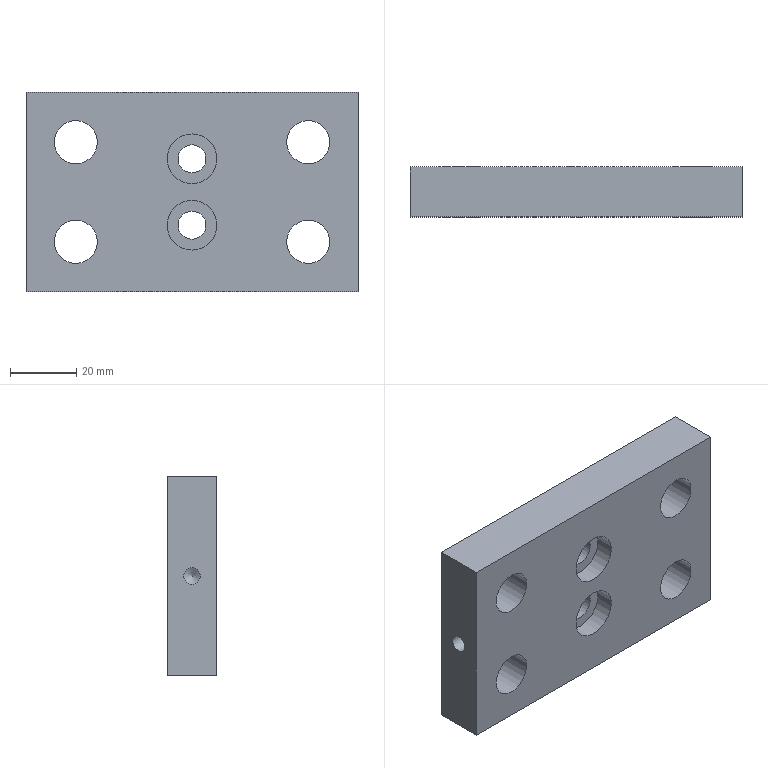Part | NX | features BREP 1 | 1 solid | 26 faces | box 100 x 15 x 60 mm | volume 77616 mm3 | cylinder 13 | plane 8 | cone 5 | commonest cylinder face diameters 13 x4 5 x3 6 x2 8.4 x2 15 x2
STEP:
#1=CARTESIAN_POINT('',(50.,-7.5,30.));
#2=VERTEX_POINT('',#1);
#3=CARTESIAN_POINT('',(50.,-7.5,-30.));
#4=VERTEX_POINT('',#3);
#5=CARTESIAN_POINT('',(50.,-7.5,30.));
#6=DIRECTION('',(0.,0.,-1.));
#7=VECTOR('',#6,1000.);
#8=LINE('',#5,#7);
#9=EDGE_CURVE('',#2,#4,#8,.T.);
#10=ORIENTED_EDGE('',*,*,#9,.T.);
#11=CARTESIAN_POINT('',(50.,7.5,-30.));
#12=VERTEX_POINT('',#11);
#13=CARTESIAN_POINT('',(50.,7.5,-30.));
#14=DIRECTION('',(0.,-1.,0.));
#15=VECTOR('',#14,1000.);
#16=LINE('',#13,#15);
#17=EDGE_CURVE('',#12,#4,#16,.T.);
#18=ORIENTED_EDGE('',*,*,#17,.F.);
#19=CARTESIAN_POINT('',(50.,7.5,30.));
#20=VERTEX_POINT('',#19);
#21=CARTESIAN_POINT('',(50.,7.5,30.));
#22=DIRECTION('',(0.,0.,-1.));
#23=VECTOR('',#22,1000.);
#24=LINE('',#21,#23);
#25=EDGE_CURVE('',#20,#12,#24,.T.);
#26=ORIENTED_EDGE('',*,*,#25,.F.);
#27=CARTESIAN_POINT('',(50.,7.5,30.));
#28=DIRECTION('',(0.,-1.,0.));
#29=VECTOR('',#28,1000.);
#30=LINE('',#27,#29);
#31=EDGE_CURVE('',#20,#2,#30,.T.);
#32=ORIENTED_EDGE('',*,*,#31,.T.);
#33=EDGE_LOOP('',(#10,#18,#26,#32));
#34=FACE_BOUND('',#33,.T.);
#35=CARTESIAN_POINT('',(50.,7.5,30.));
#36=DIRECTION('',(-1.,0.,0.));
#37=DIRECTION('',(0.,0.,-1.));
#38=AXIS2_PLACEMENT_3D('',#35,#36,#37);
#39=PLANE('',#38);
#40=ADVANCED_FACE('',(#34),#39,.F.);
#41=CARTESIAN_POINT('',(-27.5,0.,-30.));
#42=VERTEX_POINT('',#41);
#43=CARTESIAN_POINT('',(-25.,0.,-30.));
#44=DIRECTION('',(0.,0.,-1.));
#45=DIRECTION('',(-1.,0.,0.));
#46=AXIS2_PLACEMENT_3D('',#43,#44,#45);
#47=CIRCLE('',#46,2.5);
#48=EDGE_CURVE('',#42,#42,#47,.T.);
#49=ORIENTED_EDGE('',*,*,#48,.F.);
#50=EDGE_LOOP('',(#49));
#51=FACE_BOUND('',#50,.T.);
#52=CARTESIAN_POINT('',(22.5,0.,-30.));
#53=VERTEX_POINT('',#52);
#54=CARTESIAN_POINT('',(25.,0.,-30.));
#55=DIRECTION('',(0.,0.,-1.));
#56=DIRECTION('',(-1.,0.,0.));
#57=AXIS2_PLACEMENT_3D('',#54,#55,#56);
#58=CIRCLE('',#57,2.5);
#59=EDGE_CURVE('',#53,#53,#58,.T.);
#60=ORIENTED_EDGE('',*,*,#59,.F.);
#61=EDGE_LOOP('',(#60));
#62=FACE_BOUND('',#61,.T.);
#63=CARTESIAN_POINT('',(-50.,-7.5,-30.));
#64=VERTEX_POINT('',#63);
#65=CARTESIAN_POINT('',(-50.,-7.5,-30.));
#66=DIRECTION('',(-1.,0.,0.));
#67=VECTOR('',#66,1000.);
#68=LINE('',#65,#67);
#69=EDGE_CURVE('',#4,#64,#68,.T.);
#70=ORIENTED_EDGE('',*,*,#69,.T.);
#71=CARTESIAN_POINT('',(-50.,7.5,-30.));
#72=VERTEX_POINT('',#71);
#73=CARTESIAN_POINT('',(-50.,7.5,-30.));
#74=DIRECTION('',(0.,-1.,0.));
#75=VECTOR('',#74,1000.);
#76=LINE('',#73,#75);
#77=EDGE_CURVE('',#72,#64,#76,.T.);
#78=ORIENTED_EDGE('',*,*,#77,.F.);
#79=CARTESIAN_POINT('',(-50.,7.5,-30.));
#80=DIRECTION('',(-1.,0.,0.));
#81=VECTOR('',#80,1000.);
#82=LINE('',#79,#81);
#83=EDGE_CURVE('',#12,#72,#82,.T.);
#84=ORIENTED_EDGE('',*,*,#83,.F.);
#85=ORIENTED_EDGE('',*,*,#17,.T.);
#86=EDGE_LOOP('',(#70,#78,#84,#85));
#87=FACE_BOUND('',#86,.T.);
#88=CARTESIAN_POINT('',(-50.,7.5,-30.));
#89=DIRECTION('',(0.,0.,1.));
#90=DIRECTION('',(-1.,0.,0.));
#91=AXIS2_PLACEMENT_3D('',#88,#89,#90);
#92=PLANE('',#91);
#93=ADVANCED_FACE('',(#51,#62,#87),#92,.F.);
#94=CARTESIAN_POINT('',(-50.,0.,2.5));
#95=VERTEX_POINT('',#94);
#96=CARTESIAN_POINT('',(-50.,0.,0.));
#97=DIRECTION('',(-1.,0.,0.));
#98=DIRECTION('',(0.,0.,1.));
#99=AXIS2_PLACEMENT_3D('',#96,#97,#98);
#100=CIRCLE('',#99,2.5);
#101=EDGE_CURVE('',#95,#95,#100,.T.);
#102=ORIENTED_EDGE('',*,*,#101,.F.);
#103=EDGE_LOOP('',(#102));
#104=FACE_BOUND('',#103,.T.);
#105=CARTESIAN_POINT('',(-50.,-7.5,30.));
#106=VERTEX_POINT('',#105);
#107=CARTESIAN_POINT('',(-50.,-7.5,30.));
#108=DIRECTION('',(0.,0.,1.));
#109=VECTOR('',#108,1000.);
#110=LINE('',#107,#109);
#111=EDGE_CURVE('',#64,#106,#110,.T.);
#112=ORIENTED_EDGE('',*,*,#111,.T.);
#113=CARTESIAN_POINT('',(-50.,7.5,30.));
#114=VERTEX_POINT('',#113);
#115=CARTESIAN_POINT('',(-50.,7.5,30.));
#116=DIRECTION('',(0.,-1.,0.));
#117=VECTOR('',#116,1000.);
#118=LINE('',#115,#117);
#119=EDGE_CURVE('',#114,#106,#118,.T.);
#120=ORIENTED_EDGE('',*,*,#119,.F.);
#121=CARTESIAN_POINT('',(-50.,7.5,30.));
#122=DIRECTION('',(0.,0.,1.));
#123=VECTOR('',#122,1000.);
#124=LINE('',#121,#123);
#125=EDGE_CURVE('',#72,#114,#124,.T.);
#126=ORIENTED_EDGE('',*,*,#125,.F.);
#127=ORIENTED_EDGE('',*,*,#77,.T.);
#128=EDGE_LOOP('',(#112,#120,#126,#127));
#129=FACE_BOUND('',#128,.T.);
#130=CARTESIAN_POINT('',(-50.,7.5,30.));
#131=DIRECTION('',(1.,0.,0.));
#132=DIRECTION('',(0.,0.,1.));
#133=AXIS2_PLACEMENT_3D('',#130,#131,#132);
#134=PLANE('',#133);
#135=ADVANCED_FACE('',(#104,#129),#134,.F.);
#136=CARTESIAN_POINT('',(-50.,-7.5,30.));
#137=DIRECTION('',(1.,0.,0.));
#138=VECTOR('',#137,1000.);
#139=LINE('',#136,#138);
#140=EDGE_CURVE('',#106,#2,#139,.T.);
#141=ORIENTED_EDGE('',*,*,#140,.T.);
#142=ORIENTED_EDGE('',*,*,#31,.F.);
#143=CARTESIAN_POINT('',(-50.,7.5,30.));
#144=DIRECTION('',(1.,0.,0.));
#145=VECTOR('',#144,1000.);
#146=LINE('',#143,#145);
#147=EDGE_CURVE('',#114,#20,#146,.T.);
#148=ORIENTED_EDGE('',*,*,#147,.F.);
#149=ORIENTED_EDGE('',*,*,#119,.T.);
#150=EDGE_LOOP('',(#141,#142,#148,#149));
#151=FACE_BOUND('',#150,.T.);
#152=CARTESIAN_POINT('',(-50.,7.5,30.));
#153=DIRECTION('',(0.,0.,-1.));
#154=DIRECTION('',(1.,0.,0.));
#155=AXIS2_PLACEMENT_3D('',#152,#153,#154);
#156=PLANE('',#155);
#157=ADVANCED_FACE('',(#151),#156,.F.);
#158=CARTESIAN_POINT('',(-35.,7.5,-8.5));
#159=VERTEX_POINT('',#158);
#160=CARTESIAN_POINT('',(-35.,7.5,-15.));
#161=DIRECTION('',(0.,1.,0.));
#162=DIRECTION('',(0.,0.,1.));
#163=AXIS2_PLACEMENT_3D('',#160,#161,#162);
#164=CIRCLE('',#163,6.5);
#165=EDGE_CURVE('',#159,#159,#164,.T.);
#166=ORIENTED_EDGE('',*,*,#165,.F.);
#167=EDGE_LOOP('',(#166));
#168=FACE_BOUND('',#167,.T.);
#169=CARTESIAN_POINT('',(35.,7.5,21.5));
#170=VERTEX_POINT('',#169);
#171=CARTESIAN_POINT('',(35.,7.5,15.));
#172=DIRECTION('',(0.,1.,0.));
#173=DIRECTION('',(0.,0.,1.));
#174=AXIS2_PLACEMENT_3D('',#171,#172,#173);
#175=CIRCLE('',#174,6.5);
#176=EDGE_CURVE('',#170,#170,#175,.T.);
#177=ORIENTED_EDGE('',*,*,#176,.F.);
#178=EDGE_LOOP('',(#177));
#179=FACE_BOUND('',#178,.T.);
#180=CARTESIAN_POINT('',(-35.,7.5,21.5));
#181=VERTEX_POINT('',#180);
#182=CARTESIAN_POINT('',(-35.,7.5,15.));
#183=DIRECTION('',(0.,1.,0.));
#184=DIRECTION('',(0.,0.,1.));
#185=AXIS2_PLACEMENT_3D('',#182,#183,#184);
#186=CIRCLE('',#185,6.5);
#187=EDGE_CURVE('',#181,#181,#186,.T.);
#188=ORIENTED_EDGE('',*,*,#187,.F.);
#189=EDGE_LOOP('',(#188));
#190=FACE_BOUND('',#189,.T.);
#191=CARTESIAN_POINT('',(35.,7.5,-8.5));
#192=VERTEX_POINT('',#191);
#193=CARTESIAN_POINT('',(35.,7.5,-15.));
#194=DIRECTION('',(0.,1.,0.));
#195=DIRECTION('',(0.,0.,1.));
#196=AXIS2_PLACEMENT_3D('',#193,#194,#195);
#197=CIRCLE('',#196,6.5);
#198=EDGE_CURVE('',#192,#192,#197,.T.);
#199=ORIENTED_EDGE('',*,*,#198,.F.);
#200=EDGE_LOOP('',(#199));
#201=FACE_BOUND('',#200,.T.);
#202=CARTESIAN_POINT('',(0.,7.5,3.));
#203=VERTEX_POINT('',#202);
#204=CARTESIAN_POINT('',(0.,7.5,0.));
#205=DIRECTION('',(0.,1.,0.));
#206=DIRECTION('',(0.,0.,1.));
#207=AXIS2_PLACEMENT_3D('',#204,#205,#206);
#208=CIRCLE('',#207,3.);
#209=EDGE_CURVE('',#203,#203,#208,.T.);
#210=ORIENTED_EDGE('',*,*,#209,.F.);
#211=EDGE_LOOP('',(#210));
#212=FACE_BOUND('',#211,.T.);
#213=CARTESIAN_POINT('',(0.,7.5,23.));
#214=VERTEX_POINT('',#213);
#215=CARTESIAN_POINT('',(0.,7.5,20.));
#216=DIRECTION('',(0.,1.,0.));
#217=DIRECTION('',(0.,0.,1.));
#218=AXIS2_PLACEMENT_3D('',#215,#216,#217);
#219=CIRCLE('',#218,3.);
#220=EDGE_CURVE('',#214,#214,#219,.T.);
#221=ORIENTED_EDGE('',*,*,#220,.F.);
#222=EDGE_LOOP('',(#221));
#223=FACE_BOUND('',#222,.T.);
#224=CARTESIAN_POINT('',(0.,7.5,-14.2));
#225=VERTEX_POINT('',#224);
#226=CARTESIAN_POINT('',(0.,7.5,-10.));
#227=DIRECTION('',(0.,-1.,0.));
#228=DIRECTION('',(0.,0.,-1.));
#229=AXIS2_PLACEMENT_3D('',#226,#227,#228);
#230=CIRCLE('',#229,4.2);
#231=EDGE_CURVE('',#225,#225,#230,.T.);
#232=ORIENTED_EDGE('',*,*,#231,.T.);
#233=EDGE_LOOP('',(#232));
#234=FACE_BOUND('',#233,.T.);
#235=CARTESIAN_POINT('',(0.,7.5,5.8));
#236=VERTEX_POINT('',#235);
#237=CARTESIAN_POINT('',(0.,7.5,10.));
#238=DIRECTION('',(0.,-1.,0.));
#239=DIRECTION('',(0.,0.,-1.));
#240=AXIS2_PLACEMENT_3D('',#237,#238,#239);
#241=CIRCLE('',#240,4.2);
#242=EDGE_CURVE('',#236,#236,#241,.T.);
#243=ORIENTED_EDGE('',*,*,#242,.T.);
#244=EDGE_LOOP('',(#243));
#245=FACE_BOUND('',#244,.T.);
#246=ORIENTED_EDGE('',*,*,#25,.T.);
#247=ORIENTED_EDGE('',*,*,#83,.T.);
#248=ORIENTED_EDGE('',*,*,#125,.T.);
#249=ORIENTED_EDGE('',*,*,#147,.T.);
#250=EDGE_LOOP('',(#246,#247,#248,#249));
#251=FACE_BOUND('',#250,.T.);
#252=CARTESIAN_POINT('',(0.,7.5,0.));
#253=DIRECTION('',(0.,-1.,0.));
#254=DIRECTION('',(0.,0.,1.));
#255=AXIS2_PLACEMENT_3D('',#252,#253,#254);
#256=PLANE('',#255);
#257=ADVANCED_FACE('',(#168,#179,#190,#201,#212,#223,#234,#245,#251),#256,.F.);
#258=CARTESIAN_POINT('',(-35.,-7.5,-8.5));
#259=VERTEX_POINT('',#258);
#260=CARTESIAN_POINT('',(-35.,-7.5,-15.));
#261=DIRECTION('',(0.,1.,0.));
#262=DIRECTION('',(0.,0.,1.));
#263=AXIS2_PLACEMENT_3D('',#260,#261,#262);
#264=CIRCLE('',#263,6.5);
#265=EDGE_CURVE('',#259,#259,#264,.T.);
#266=ORIENTED_EDGE('',*,*,#265,.T.);
#267=EDGE_LOOP('',(#266));
#268=FACE_BOUND('',#267,.T.);
#269=CARTESIAN_POINT('',(35.,-7.5,21.5));
#270=VERTEX_POINT('',#269);
#271=CARTESIAN_POINT('',(35.,-7.5,15.));
#272=DIRECTION('',(0.,1.,0.));
#273=DIRECTION('',(0.,0.,1.));
#274=AXIS2_PLACEMENT_3D('',#271,#272,#273);
#275=CIRCLE('',#274,6.5);
#276=EDGE_CURVE('',#270,#270,#275,.T.);
#277=ORIENTED_EDGE('',*,*,#276,.T.);
#278=EDGE_LOOP('',(#277));
#279=FACE_BOUND('',#278,.T.);
#280=CARTESIAN_POINT('',(-35.,-7.5,21.5));
#281=VERTEX_POINT('',#280);
#282=CARTESIAN_POINT('',(-35.,-7.5,15.));
#283=DIRECTION('',(0.,1.,0.));
#284=DIRECTION('',(0.,0.,1.));
#285=AXIS2_PLACEMENT_3D('',#282,#283,#284);
#286=CIRCLE('',#285,6.5);
#287=EDGE_CURVE('',#281,#281,#286,.T.);
#288=ORIENTED_EDGE('',*,*,#287,.T.);
#289=EDGE_LOOP('',(#288));
#290=FACE_BOUND('',#289,.T.);
#291=CARTESIAN_POINT('',(35.,-7.5,-8.5));
#292=VERTEX_POINT('',#291);
#293=CARTESIAN_POINT('',(35.,-7.5,-15.));
#294=DIRECTION('',(0.,1.,0.));
#295=DIRECTION('',(0.,0.,1.));
#296=AXIS2_PLACEMENT_3D('',#293,#294,#295);
#297=CIRCLE('',#296,6.5);
#298=EDGE_CURVE('',#292,#292,#297,.T.);
#299=ORIENTED_EDGE('',*,*,#298,.T.);
#300=EDGE_LOOP('',(#299));
#301=FACE_BOUND('',#300,.T.);
#302=CARTESIAN_POINT('',(0.,-7.5,-17.5));
#303=VERTEX_POINT('',#302);
#304=CARTESIAN_POINT('',(0.,-7.5,-10.));
#305=DIRECTION('',(0.,-1.,0.));
#306=DIRECTION('',(0.,0.,-1.));
#307=AXIS2_PLACEMENT_3D('',#304,#305,#306);
#308=CIRCLE('',#307,7.5);
#309=EDGE_CURVE('',#303,#303,#308,.T.);
#310=ORIENTED_EDGE('',*,*,#309,.F.);
#311=EDGE_LOOP('',(#310));
#312=FACE_BOUND('',#311,.T.);
#313=CARTESIAN_POINT('',(0.,-7.5,2.5));
#314=VERTEX_POINT('',#313);
#315=CARTESIAN_POINT('',(0.,-7.5,10.));
#316=DIRECTION('',(0.,-1.,0.));
#317=DIRECTION('',(0.,0.,-1.));
#318=AXIS2_PLACEMENT_3D('',#315,#316,#317);
#319=CIRCLE('',#318,7.5);
#320=EDGE_CURVE('',#314,#314,#319,.T.);
#321=ORIENTED_EDGE('',*,*,#320,.F.);
#322=EDGE_LOOP('',(#321));
#323=FACE_BOUND('',#322,.T.);
#324=ORIENTED_EDGE('',*,*,#9,.F.);
#325=ORIENTED_EDGE('',*,*,#140,.F.);
#326=ORIENTED_EDGE('',*,*,#111,.F.);
#327=ORIENTED_EDGE('',*,*,#69,.F.);
#328=EDGE_LOOP('',(#324,#325,#326,#327));
#329=FACE_BOUND('',#328,.T.);
#330=CARTESIAN_POINT('',(0.,-7.5,0.));
#331=DIRECTION('',(0.,-1.,0.));
#332=DIRECTION('',(0.,0.,1.));
#333=AXIS2_PLACEMENT_3D('',#330,#331,#332);
#334=PLANE('',#333);
#335=ADVANCED_FACE('',(#268,#279,#290,#301,#312,#323,#329),#334,.T.);
#336=ORIENTED_EDGE('',*,*,#242,.F.);
#337=EDGE_LOOP('',(#336));
#338=FACE_BOUND('',#337,.T.);
#339=CARTESIAN_POINT('',(0.,-1.9,5.8));
#340=VERTEX_POINT('',#339);
#341=CARTESIAN_POINT('',(0.,-1.9,10.));
#342=DIRECTION('',(0.,-1.,0.));
#343=DIRECTION('',(0.,0.,-1.));
#344=AXIS2_PLACEMENT_3D('',#341,#342,#343);
#345=CIRCLE('',#344,4.2);
#346=EDGE_CURVE('',#340,#340,#345,.T.);
#347=ORIENTED_EDGE('',*,*,#346,.T.);
#348=EDGE_LOOP('',(#347));
#349=FACE_BOUND('',#348,.T.);
#350=CARTESIAN_POINT('',(0.,-7.5,10.));
#351=DIRECTION('',(0.,-1.,0.));
#352=DIRECTION('',(0.,0.,1.));
#353=AXIS2_PLACEMENT_3D('',#350,#351,#352);
#354=CYLINDRICAL_SURFACE('',#353,4.2);
#355=ADVANCED_FACE('',(#338,#349),#354,.F.);
#356=ORIENTED_EDGE('',*,*,#346,.F.);
#357=EDGE_LOOP('',(#356));
#358=FACE_BOUND('',#357,.T.);
#359=CARTESIAN_POINT('',(0.,-1.9,2.5));
#360=VERTEX_POINT('',#359);
#361=CARTESIAN_POINT('',(0.,-1.9,10.));
#362=DIRECTION('',(0.,-1.,0.));
#363=DIRECTION('',(0.,0.,-1.));
#364=AXIS2_PLACEMENT_3D('',#361,#362,#363);
#365=CIRCLE('',#364,7.5);
#366=EDGE_CURVE('',#360,#360,#365,.T.);
#367=ORIENTED_EDGE('',*,*,#366,.T.);
#368=EDGE_LOOP('',(#367));
#369=FACE_BOUND('',#368,.T.);
#370=CARTESIAN_POINT('',(4.2,-1.9,10.));
#371=DIRECTION('',(0.,1.,0.));
#372=DIRECTION('',(0.,0.,-1.));
#373=AXIS2_PLACEMENT_3D('',#370,#371,#372);
#374=PLANE('',#373);
#375=ADVANCED_FACE('',(#358,#369),#374,.F.);
#376=ORIENTED_EDGE('',*,*,#366,.F.);
#377=EDGE_LOOP('',(#376));
#378=FACE_BOUND('',#377,.T.);
#379=ORIENTED_EDGE('',*,*,#320,.T.);
#380=EDGE_LOOP('',(#379));
#381=FACE_BOUND('',#380,.T.);
#382=CARTESIAN_POINT('',(0.,-7.5,10.));
#383=DIRECTION('',(0.,-1.,0.));
#384=DIRECTION('',(0.,0.,1.));
#385=AXIS2_PLACEMENT_3D('',#382,#383,#384);
#386=CYLINDRICAL_SURFACE('',#385,7.5);
#387=ADVANCED_FACE('',(#378,#381),#386,.F.);
#388=ORIENTED_EDGE('',*,*,#231,.F.);
#389=EDGE_LOOP('',(#388));
#390=FACE_BOUND('',#389,.T.);
#391=CARTESIAN_POINT('',(0.,-1.9,-14.2));
#392=VERTEX_POINT('',#391);
#393=CARTESIAN_POINT('',(0.,-1.9,-10.));
#394=DIRECTION('',(0.,-1.,0.));
#395=DIRECTION('',(0.,0.,-1.));
#396=AXIS2_PLACEMENT_3D('',#393,#394,#395);
#397=CIRCLE('',#396,4.2);
#398=EDGE_CURVE('',#392,#392,#397,.T.);
#399=ORIENTED_EDGE('',*,*,#398,.T.);
#400=EDGE_LOOP('',(#399));
#401=FACE_BOUND('',#400,.T.);
#402=CARTESIAN_POINT('',(0.,-7.5,-10.));
#403=DIRECTION('',(0.,-1.,0.));
#404=DIRECTION('',(0.,0.,1.));
#405=AXIS2_PLACEMENT_3D('',#402,#403,#404);
#406=CYLINDRICAL_SURFACE('',#405,4.2);
#407=ADVANCED_FACE('',(#390,#401),#406,.F.);
#408=ORIENTED_EDGE('',*,*,#398,.F.);
#409=EDGE_LOOP('',(#408));
#410=FACE_BOUND('',#409,.T.);
#411=CARTESIAN_POINT('',(0.,-1.9,-17.5));
#412=VERTEX_POINT('',#411);
#413=CARTESIAN_POINT('',(0.,-1.9,-10.));
#414=DIRECTION('',(0.,-1.,0.));
#415=DIRECTION('',(0.,0.,-1.));
#416=AXIS2_PLACEMENT_3D('',#413,#414,#415);
#417=CIRCLE('',#416,7.5);
#418=EDGE_CURVE('',#412,#412,#417,.T.);
#419=ORIENTED_EDGE('',*,*,#418,.T.);
#420=EDGE_LOOP('',(#419));
#421=FACE_BOUND('',#420,.T.);
#422=CARTESIAN_POINT('',(4.2,-1.9,-10.));
#423=DIRECTION('',(0.,1.,0.));
#424=DIRECTION('',(0.,0.,-1.));
#425=AXIS2_PLACEMENT_3D('',#422,#423,#424);
#426=PLANE('',#425);
#427=ADVANCED_FACE('',(#410,#421),#426,.F.);
#428=ORIENTED_EDGE('',*,*,#418,.F.);
#429=EDGE_LOOP('',(#428));
#430=FACE_BOUND('',#429,.T.);
#431=ORIENTED_EDGE('',*,*,#309,.T.);
#432=EDGE_LOOP('',(#431));
#433=FACE_BOUND('',#432,.T.);
#434=CARTESIAN_POINT('',(0.,-7.5,-10.));
#435=DIRECTION('',(0.,-1.,0.));
#436=DIRECTION('',(0.,0.,1.));
#437=AXIS2_PLACEMENT_3D('',#434,#435,#436);
#438=CYLINDRICAL_SURFACE('',#437,7.5);
#439=ADVANCED_FACE('',(#430,#433),#438,.F.);
#440=CARTESIAN_POINT('',(0.,-2.303,20.));
#441=VERTEX_POINT('',#440);
#442=VERTEX_LOOP('',#441);
#443=FACE_BOUND('',#442,.T.);
#444=CARTESIAN_POINT('',(0.,-0.5,23.));
#445=VERTEX_POINT('',#444);
#446=CARTESIAN_POINT('',(0.,-0.5,20.));
#447=DIRECTION('',(0.,1.,0.));
#448=DIRECTION('',(0.,0.,1.));
#449=AXIS2_PLACEMENT_3D('',#446,#447,#448);
#450=CIRCLE('',#449,3.);
#451=EDGE_CURVE('',#445,#445,#450,.T.);
#452=ORIENTED_EDGE('',*,*,#451,.T.);
#453=EDGE_LOOP('',(#452));
#454=FACE_BOUND('',#453,.T.);
#455=CARTESIAN_POINT('',(0.,-0.5,20.));
#456=DIRECTION('',(0.,1.,0.));
#457=DIRECTION('',(0.,0.,-1.));
#458=AXIS2_PLACEMENT_3D('',#455,#456,#457);
#459=CONICAL_SURFACE('',#458,3.,1.03);
#460=ADVANCED_FACE('',(#443,#454),#459,.F.);
#461=ORIENTED_EDGE('',*,*,#451,.F.);
#462=EDGE_LOOP('',(#461));
#463=FACE_BOUND('',#462,.T.);
#464=ORIENTED_EDGE('',*,*,#220,.T.);
#465=EDGE_LOOP('',(#464));
#466=FACE_BOUND('',#465,.T.);
#467=CARTESIAN_POINT('',(0.,7.5,20.));
#468=DIRECTION('',(0.,1.,0.));
#469=DIRECTION('',(0.,0.,-1.));
#470=AXIS2_PLACEMENT_3D('',#467,#468,#469);
#471=CYLINDRICAL_SURFACE('',#470,3.);
#472=ADVANCED_FACE('',(#463,#466),#471,.F.);
#473=CARTESIAN_POINT('',(0.,-2.303,0.));
#474=VERTEX_POINT('',#473);
#475=VERTEX_LOOP('',#474);
#476=FACE_BOUND('',#475,.T.);
#477=CARTESIAN_POINT('',(0.,-0.5,3.));
#478=VERTEX_POINT('',#477);
#479=CARTESIAN_POINT('',(0.,-0.5,0.));
#480=DIRECTION('',(0.,1.,0.));
#481=DIRECTION('',(0.,0.,1.));
#482=AXIS2_PLACEMENT_3D('',#479,#480,#481);
#483=CIRCLE('',#482,3.);
#484=EDGE_CURVE('',#478,#478,#483,.T.);
#485=ORIENTED_EDGE('',*,*,#484,.T.);
#486=EDGE_LOOP('',(#485));
#487=FACE_BOUND('',#486,.T.);
#488=CARTESIAN_POINT('',(0.,-0.5,0.));
#489=DIRECTION('',(0.,1.,0.));
#490=DIRECTION('',(0.,0.,-1.));
#491=AXIS2_PLACEMENT_3D('',#488,#489,#490);
#492=CONICAL_SURFACE('',#491,3.,1.03);
#493=ADVANCED_FACE('',(#476,#487),#492,.F.);
#494=ORIENTED_EDGE('',*,*,#484,.F.);
#495=EDGE_LOOP('',(#494));
#496=FACE_BOUND('',#495,.T.);
#497=ORIENTED_EDGE('',*,*,#209,.T.);
#498=EDGE_LOOP('',(#497));
#499=FACE_BOUND('',#498,.T.);
#500=CARTESIAN_POINT('',(0.,7.5,0.));
#501=DIRECTION('',(0.,1.,0.));
#502=DIRECTION('',(0.,0.,-1.));
#503=AXIS2_PLACEMENT_3D('',#500,#501,#502);
#504=CYLINDRICAL_SURFACE('',#503,3.);
#505=ADVANCED_FACE('',(#496,#499),#504,.F.);
#506=ORIENTED_EDGE('',*,*,#298,.F.);
#507=EDGE_LOOP('',(#506));
#508=FACE_BOUND('',#507,.T.);
#509=ORIENTED_EDGE('',*,*,#198,.T.);
#510=EDGE_LOOP('',(#509));
#511=FACE_BOUND('',#510,.T.);
#512=CARTESIAN_POINT('',(35.,7.5,-15.));
#513=DIRECTION('',(0.,1.,0.));
#514=DIRECTION('',(0.,0.,-1.));
#515=AXIS2_PLACEMENT_3D('',#512,#513,#514);
#516=CYLINDRICAL_SURFACE('',#515,6.5);
#517=ADVANCED_FACE('',(#508,#511),#516,.F.);
#518=ORIENTED_EDGE('',*,*,#287,.F.);
#519=EDGE_LOOP('',(#518));
#520=FACE_BOUND('',#519,.T.);
#521=ORIENTED_EDGE('',*,*,#187,.T.);
#522=EDGE_LOOP('',(#521));
#523=FACE_BOUND('',#522,.T.);
#524=CARTESIAN_POINT('',(-35.,7.5,15.));
#525=DIRECTION('',(0.,1.,0.));
#526=DIRECTION('',(0.,0.,-1.));
#527=AXIS2_PLACEMENT_3D('',#524,#525,#526);
#528=CYLINDRICAL_SURFACE('',#527,6.5);
#529=ADVANCED_FACE('',(#520,#523),#528,.F.);
#530=ORIENTED_EDGE('',*,*,#276,.F.);
#531=EDGE_LOOP('',(#530));
#532=FACE_BOUND('',#531,.T.);
#533=ORIENTED_EDGE('',*,*,#176,.T.);
#534=EDGE_LOOP('',(#533));
#535=FACE_BOUND('',#534,.T.);
#536=CARTESIAN_POINT('',(35.,7.5,15.));
#537=DIRECTION('',(0.,1.,0.));
#538=DIRECTION('',(0.,0.,-1.));
#539=AXIS2_PLACEMENT_3D('',#536,#537,#538);
#540=CYLINDRICAL_SURFACE('',#539,6.5);
#541=ADVANCED_FACE('',(#532,#535),#540,.F.);
#542=ORIENTED_EDGE('',*,*,#265,.F.);
#543=EDGE_LOOP('',(#542));
#544=FACE_BOUND('',#543,.T.);
#545=ORIENTED_EDGE('',*,*,#165,.T.);
#546=EDGE_LOOP('',(#545));
#547=FACE_BOUND('',#546,.T.);
#548=CARTESIAN_POINT('',(-35.,7.5,-15.));
#549=DIRECTION('',(0.,1.,0.));
#550=DIRECTION('',(0.,0.,-1.));
#551=AXIS2_PLACEMENT_3D('',#548,#549,#550);
#552=CYLINDRICAL_SURFACE('',#551,6.5);
#553=ADVANCED_FACE('',(#544,#547),#552,.F.);
#554=CARTESIAN_POINT('',(25.,0.,-13.498));
#555=VERTEX_POINT('',#554);
#556=VERTEX_LOOP('',#555);
#557=FACE_BOUND('',#556,.T.);
#558=CARTESIAN_POINT('',(22.5,0.,-15.));
#559=VERTEX_POINT('',#558);
#560=CARTESIAN_POINT('',(25.,0.,-15.));
#561=DIRECTION('',(0.,0.,-1.));
#562=DIRECTION('',(-1.,0.,0.));
#563=AXIS2_PLACEMENT_3D('',#560,#561,#562);
#564=CIRCLE('',#563,2.5);
#565=EDGE_CURVE('',#559,#559,#564,.T.);
#566=ORIENTED_EDGE('',*,*,#565,.T.);
#567=EDGE_LOOP('',(#566));
#568=FACE_BOUND('',#567,.T.);
#569=CARTESIAN_POINT('',(25.,0.,-15.));
#570=DIRECTION('',(0.,0.,-1.));
#571=DIRECTION('',(1.,0.,0.));
#572=AXIS2_PLACEMENT_3D('',#569,#570,#571);
#573=CONICAL_SURFACE('',#572,2.5,1.03);
#574=ADVANCED_FACE('',(#557,#568),#573,.F.);
#575=ORIENTED_EDGE('',*,*,#565,.F.);
#576=EDGE_LOOP('',(#575));
#577=FACE_BOUND('',#576,.T.);
#578=ORIENTED_EDGE('',*,*,#59,.T.);
#579=EDGE_LOOP('',(#578));
#580=FACE_BOUND('',#579,.T.);
#581=CARTESIAN_POINT('',(25.,0.,-30.));
#582=DIRECTION('',(0.,0.,-1.));
#583=DIRECTION('',(1.,0.,0.));
#584=AXIS2_PLACEMENT_3D('',#581,#582,#583);
#585=CYLINDRICAL_SURFACE('',#584,2.5);
#586=ADVANCED_FACE('',(#577,#580),#585,.F.);
#587=CARTESIAN_POINT('',(-25.,0.,-13.498));
#588=VERTEX_POINT('',#587);
#589=VERTEX_LOOP('',#588);
#590=FACE_BOUND('',#589,.T.);
#591=CARTESIAN_POINT('',(-27.5,0.,-15.));
#592=VERTEX_POINT('',#591);
#593=CARTESIAN_POINT('',(-25.,0.,-15.));
#594=DIRECTION('',(0.,0.,-1.));
#595=DIRECTION('',(-1.,0.,0.));
#596=AXIS2_PLACEMENT_3D('',#593,#594,#595);
#597=CIRCLE('',#596,2.5);
#598=EDGE_CURVE('',#592,#592,#597,.T.);
#599=ORIENTED_EDGE('',*,*,#598,.T.);
#600=EDGE_LOOP('',(#599));
#601=FACE_BOUND('',#600,.T.);
#602=CARTESIAN_POINT('',(-25.,0.,-15.));
#603=DIRECTION('',(0.,0.,-1.));
#604=DIRECTION('',(1.,0.,0.));
#605=AXIS2_PLACEMENT_3D('',#602,#603,#604);
#606=CONICAL_SURFACE('',#605,2.5,1.03);
#607=ADVANCED_FACE('',(#590,#601),#606,.F.);
#608=ORIENTED_EDGE('',*,*,#598,.F.);
#609=EDGE_LOOP('',(#608));
#610=FACE_BOUND('',#609,.T.);
#611=ORIENTED_EDGE('',*,*,#48,.T.);
#612=EDGE_LOOP('',(#611));
#613=FACE_BOUND('',#612,.T.);
#614=CARTESIAN_POINT('',(-25.,0.,-30.));
#615=DIRECTION('',(0.,0.,-1.));
#616=DIRECTION('',(1.,0.,0.));
#617=AXIS2_PLACEMENT_3D('',#614,#615,#616);
#618=CYLINDRICAL_SURFACE('',#617,2.5);
#619=ADVANCED_FACE('',(#610,#613),#618,.F.);
#620=CARTESIAN_POINT('',(-33.498,0.,0.));
#621=VERTEX_POINT('',#620);
#622=VERTEX_LOOP('',#621);
#623=FACE_BOUND('',#622,.T.);
#624=CARTESIAN_POINT('',(-35.,0.,2.5));
#625=VERTEX_POINT('',#624);
#626=CARTESIAN_POINT('',(-35.,0.,0.));
#627=DIRECTION('',(-1.,0.,0.));
#628=DIRECTION('',(0.,0.,1.));
#629=AXIS2_PLACEMENT_3D('',#626,#627,#628);
#630=CIRCLE('',#629,2.5);
#631=EDGE_CURVE('',#625,#625,#630,.T.);
#632=ORIENTED_EDGE('',*,*,#631,.T.);
#633=EDGE_LOOP('',(#632));
#634=FACE_BOUND('',#633,.T.);
#635=CARTESIAN_POINT('',(-35.,0.,0.));
#636=DIRECTION('',(-1.,0.,0.));
#637=DIRECTION('',(0.,0.,-1.));
#638=AXIS2_PLACEMENT_3D('',#635,#636,#637);
#639=CONICAL_SURFACE('',#638,2.5,1.03);
#640=ADVANCED_FACE('',(#623,#634),#639,.F.);
#641=ORIENTED_EDGE('',*,*,#631,.F.);
#642=EDGE_LOOP('',(#641));
#643=FACE_BOUND('',#642,.T.);
#644=ORIENTED_EDGE('',*,*,#101,.T.);
#645=EDGE_LOOP('',(#644));
#646=FACE_BOUND('',#645,.T.);
#647=CARTESIAN_POINT('',(-50.,0.,0.));
#648=DIRECTION('',(-1.,0.,0.));
#649=DIRECTION('',(0.,0.,-1.));
#650=AXIS2_PLACEMENT_3D('',#647,#648,#649);
#651=CYLINDRICAL_SURFACE('',#650,2.5);
#652=ADVANCED_FACE('',(#643,#646),#651,.F.);
#653=CLOSED_SHELL('',(#40,#93,#135,#157,#257,#335,#355,#375,#387,#407,#427,#439,#460,#472,#493,#505,#517,#529,#541,#553,#574,#586,#607,#619,#640,#652));
#654=MANIFOLD_SOLID_BREP('',#653);
#655=(LENGTH_UNIT()NAMED_UNIT(*)SI_UNIT(.MILLI.,.METRE.));
#656=UNCERTAINTY_MEASURE_WITH_UNIT(LENGTH_MEASURE(0.00001),#655,'','');
#657=(NAMED_UNIT(*)PLANE_ANGLE_UNIT()SI_UNIT($,.RADIAN.));
#658=(NAMED_UNIT(*)SI_UNIT($,.STERADIAN.)SOLID_ANGLE_UNIT());
#659=(GEOMETRIC_REPRESENTATION_CONTEXT(3)GLOBAL_UNCERTAINTY_ASSIGNED_CONTEXT((#656))GLOBAL_UNIT_ASSIGNED_CONTEXT((#655,#657,#658))REPRESENTATION_CONTEXT('',''));
#660=ADVANCED_BREP_SHAPE_REPRESENTATION('',(#654),#659);